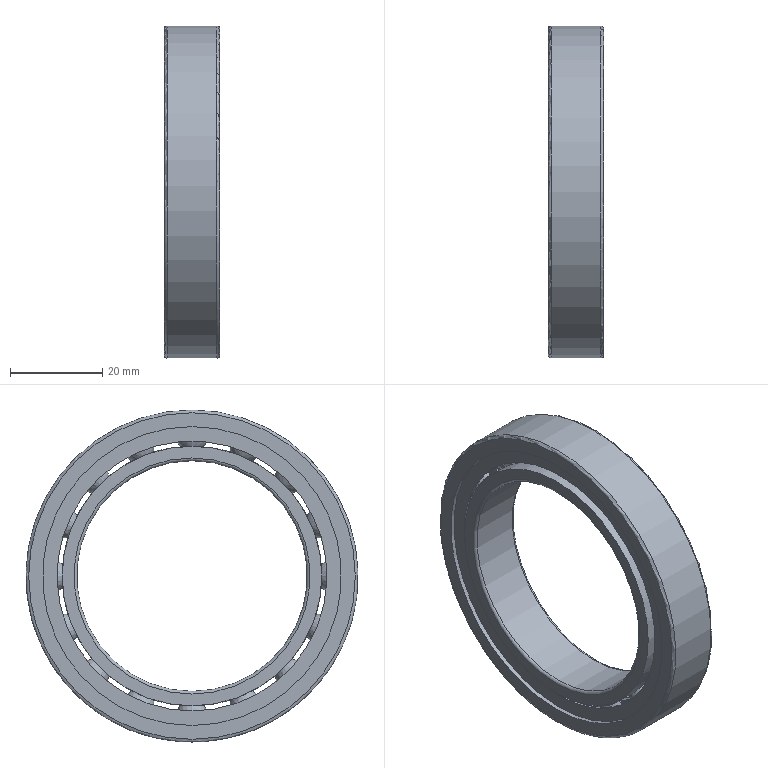Part | NX | features BREP 1 | 1 solid | 152 faces | box 12 x 72 x 72 mm | volume 17492 mm3 | sphere 64 | plane 40 | torus 36 | cylinder 12 | commonest cylinder face diameters 64.8 x4 56.3 x2 58.527 x2 50 x1 58.695 x1 62.405 x1